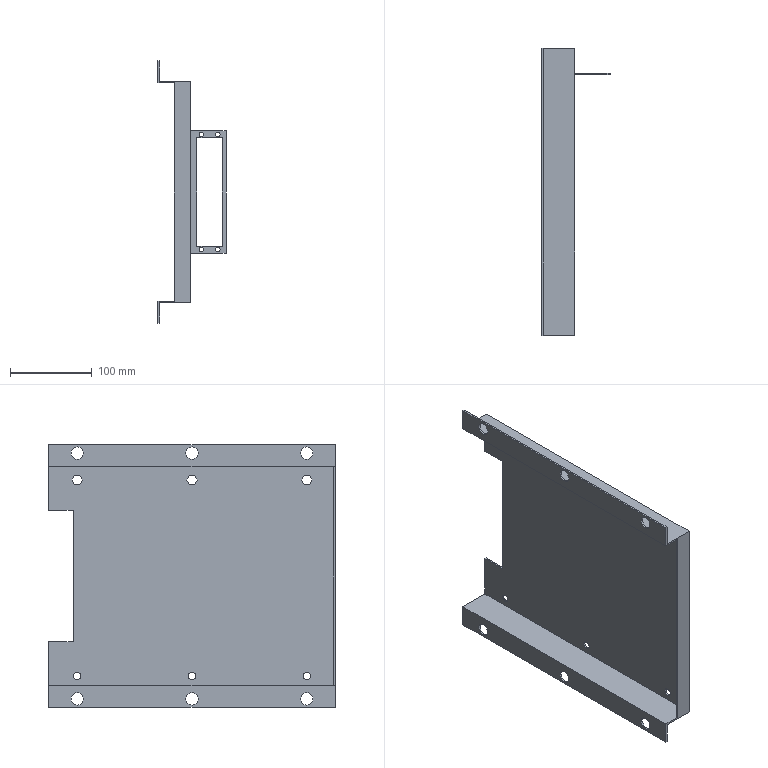Part | SolidWorks | features BaseBody 1 | 1 solid | 72 faces | box 83 x 350 x 320 mm | volume 278562 mm3 | plane 46 | cylinder 26 | commonest cylinder face diameters 15 x12 5.5 x8 9.1 x6